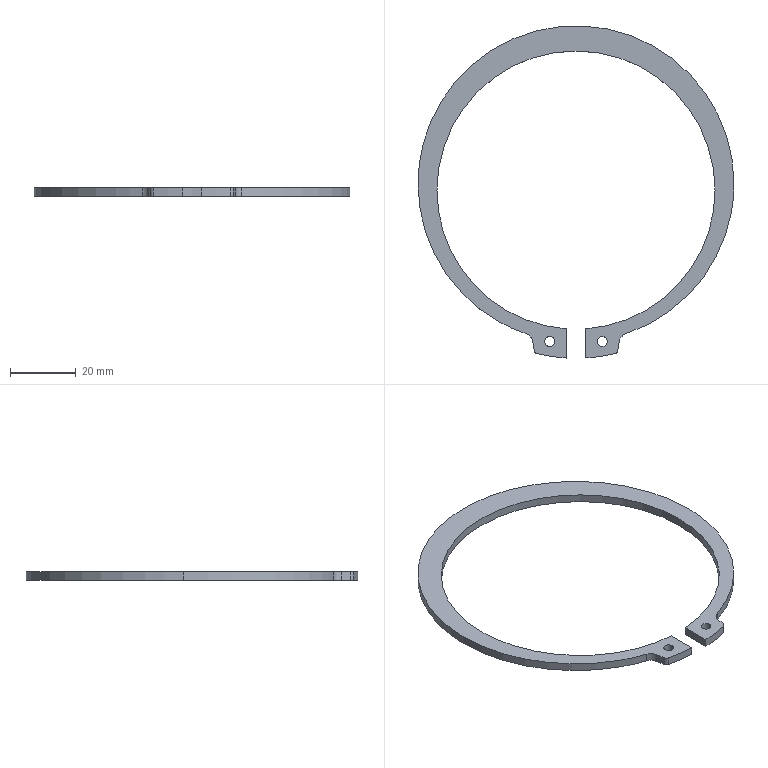Part | STEP file | PN_0045_Default<As Machined> | 1 solid | 22 faces | box 96 x 100.912 x 2.5 mm | volume 4237 mm3 | cylinder 16 | plane 6 | commonest cylinder face diameters 3 x4 84.5 x3 96 x3 2.4 x2 6 x2 102.2 x2
STEP:
#1=CARTESIAN_POINT('',(6.5,-47.91,-2.5));
#2=VERTEX_POINT('',#1);
#3=CARTESIAN_POINT('',(9.5,-47.91,-2.5));
#4=VERTEX_POINT('',#3);
#5=CARTESIAN_POINT('',(8.,-47.91,-2.5));
#6=DIRECTION('',(0.,0.,1.));
#7=AXIS2_PLACEMENT_3D('',#5,#6,$);
#8=CIRCLE('',#7,1.5);
#9=EDGE_CURVE('',#2,#4,#8,.T.);
#10=ORIENTED_EDGE('',*,*,#9,.F.);
#11=CARTESIAN_POINT('',(6.5,-47.91,0.));
#12=VERTEX_POINT('',#11);
#13=CARTESIAN_POINT('',(6.5,-47.91,-2.5));
#14=DIRECTION('',(0.,0.,1.));
#15=VECTOR('',#14,1.);
#16=LINE('',#13,#15);
#17=EDGE_CURVE('',#2,#12,#16,.T.);
#18=ORIENTED_EDGE('',*,*,#17,.T.);
#19=CARTESIAN_POINT('',(9.5,-47.91,0.));
#20=VERTEX_POINT('',#19);
#21=CARTESIAN_POINT('',(8.,-47.91,0.));
#22=DIRECTION('',(0.,0.,1.));
#23=AXIS2_PLACEMENT_3D('',#21,#22,$);
#24=CIRCLE('',#23,1.5);
#25=EDGE_CURVE('',#12,#20,#24,.T.);
#26=ORIENTED_EDGE('',*,*,#25,.T.);
#27=CARTESIAN_POINT('',(9.5,-47.91,-2.5));
#28=DIRECTION('',(0.,0.,1.));
#29=VECTOR('',#28,1.);
#30=LINE('',#27,#29);
#31=EDGE_CURVE('',#4,#20,#30,.T.);
#32=ORIENTED_EDGE('',*,*,#31,.F.);
#33=EDGE_LOOP('',(#10,#18,#26,#32));
#34=FACE_OUTER_BOUND('',#33,.T.);
#35=CARTESIAN_POINT('',(8.,-47.91,-2.5));
#36=DIRECTION('',(0.,0.,1.));
#37=DIRECTION('',(-1.,0.,0.));
#38=AXIS2_PLACEMENT_3D('',#35,#36,#37);
#39=CYLINDRICAL_SURFACE('',#38,1.5);
#40=ADVANCED_FACE('',(#34),#39,.F.);
#41=CARTESIAN_POINT('',(-11.757,-51.629,-2.5));
#42=VERTEX_POINT('',#41);
#43=CARTESIAN_POINT('',(-3.,-52.912,-2.5));
#44=VERTEX_POINT('',#43);
#45=CARTESIAN_POINT('',(-11.757,-51.629,-2.5));
#46=CARTESIAN_POINT('',(-10.032,-52.037,-2.5));
#47=CARTESIAN_POINT('',(-8.29,-52.37,-2.5));
#48=CARTESIAN_POINT('',(-6.534,-52.627,-2.5));
#49=CARTESIAN_POINT('',(-4.769,-52.808,-2.5));
#50=CARTESIAN_POINT('',(-3.,-52.912,-2.5));
#51=B_SPLINE_CURVE_WITH_KNOTS('',5,(#45,#46,#47,#48,#49,#50),.UNSPECIFIED.,.F.,.U.,(6,6),(0.,12.532),.UNSPECIFIED.);
#52=EDGE_CURVE('',#42,#44,#51,.T.);
#53=ORIENTED_EDGE('',*,*,#52,.F.);
#54=CARTESIAN_POINT('',(-12.662,-50.67,-2.5));
#55=VERTEX_POINT('',#54);
#56=CARTESIAN_POINT('',(-11.481,-50.461,-2.5));
#57=DIRECTION('',(0.,0.,-1.));
#58=AXIS2_PLACEMENT_3D('',#56,#57,$);
#59=CIRCLE('',#58,1.2);
#60=EDGE_CURVE('',#42,#55,#59,.T.);
#61=ORIENTED_EDGE('',*,*,#60,.T.);
#62=CARTESIAN_POINT('',(-13.157,-47.867,-2.5));
#63=VERTEX_POINT('',#62);
#64=CARTESIAN_POINT('',(-12.91,-49.269,-2.5));
#65=DIRECTION('',(0.1736,-0.9848,0.));
#66=VECTOR('',#65,1.);
#67=LINE('',#64,#66);
#68=EDGE_CURVE('',#63,#55,#67,.T.);
#69=ORIENTED_EDGE('',*,*,#68,.F.);
#70=CARTESIAN_POINT('',(-15.163,-45.542,-2.5));
#71=VERTEX_POINT('',#70);
#72=CARTESIAN_POINT('',(-13.157,-47.867,-2.5));
#73=CARTESIAN_POINT('',(-13.216,-47.533,-2.5));
#74=CARTESIAN_POINT('',(-13.322,-47.207,-2.5));
#75=CARTESIAN_POINT('',(-13.474,-46.899,-2.5));
#76=CARTESIAN_POINT('',(-13.841,-46.361,-2.5));
#77=CARTESIAN_POINT('',(-14.337,-45.94,-2.5));
#78=CARTESIAN_POINT('',(-14.596,-45.772,-2.5));
#79=CARTESIAN_POINT('',(-14.873,-45.639,-2.5));
#80=CARTESIAN_POINT('',(-15.163,-45.542,-2.5));
#81=B_SPLINE_CURVE_WITH_KNOTS('',5,(#72,#73,#74,#75,#76,#77,#78,#79,#80),.UNSPECIFIED.,.F.,.U.,(6,3,6),(0.,2.4,4.56),.UNSPECIFIED.);
#82=EDGE_CURVE('',#63,#71,#81,.T.);
#83=ORIENTED_EDGE('',*,*,#82,.T.);
#84=CARTESIAN_POINT('',(-48.,0.,-2.5));
#85=VERTEX_POINT('',#84);
#86=CARTESIAN_POINT('',(-48.,0.,-2.5));
#87=CARTESIAN_POINT('',(-48.,-4.412,-2.5));
#88=CARTESIAN_POINT('',(-47.493,-8.825,-2.5));
#89=CARTESIAN_POINT('',(-46.479,-13.159,-2.5));
#90=CARTESIAN_POINT('',(-43.473,-21.518,-2.5));
#91=CARTESIAN_POINT('',(-38.65,-28.977,-2.5));
#92=CARTESIAN_POINT('',(-35.818,-32.412,-2.5));
#93=CARTESIAN_POINT('',(-30.318,-37.703,-2.5));
#94=CARTESIAN_POINT('',(-23.91,-41.803,-2.5));
#95=CARTESIAN_POINT('',(-21.095,-43.291,-2.5));
#96=CARTESIAN_POINT('',(-18.17,-44.541,-2.5));
#97=CARTESIAN_POINT('',(-15.163,-45.542,-2.5));
#98=B_SPLINE_CURVE_WITH_KNOTS('',5,(#86,#87,#88,#89,#90,#91,#92,#93,#94,#95,#96,#97),.UNSPECIFIED.,.F.,.U.,(6,3,3,6),(0.,31.2,62.399,84.811),.UNSPECIFIED.);
#99=EDGE_CURVE('',#85,#71,#98,.T.);
#100=ORIENTED_EDGE('',*,*,#99,.F.);
#101=CARTESIAN_POINT('',(48.,0.,-2.5));
#102=VERTEX_POINT('',#101);
#103=CARTESIAN_POINT('',(48.,0.,-2.5));
#104=CARTESIAN_POINT('',(48.,4.412,-2.5));
#105=CARTESIAN_POINT('',(47.493,8.825,-2.5));
#106=CARTESIAN_POINT('',(46.479,13.159,-2.5));
#107=CARTESIAN_POINT('',(43.473,21.518,-2.5));
#108=CARTESIAN_POINT('',(38.65,28.977,-2.5));
#109=CARTESIAN_POINT('',(35.818,32.412,-2.5));
#110=CARTESIAN_POINT('',(29.416,38.57,-2.5));
#111=CARTESIAN_POINT('',(21.784,43.115,-2.5));
#112=CARTESIAN_POINT('',(17.722,44.937,-2.5));
#113=CARTESIAN_POINT('',(9.253,47.616,-2.5));
#114=CARTESIAN_POINT('',(0.3973,48.304,-2.5));
#115=CARTESIAN_POINT('',(-4.051,48.136,-2.5));
#116=CARTESIAN_POINT('',(-12.83,46.78,-2.5));
#117=CARTESIAN_POINT('',(-21.072,43.468,-2.5));
#118=CARTESIAN_POINT('',(-24.984,41.343,-2.5));
#119=CARTESIAN_POINT('',(-32.25,36.233,-2.5));
#120=CARTESIAN_POINT('',(-38.168,29.609,-2.5));
#121=CARTESIAN_POINT('',(-40.731,25.969,-2.5));
#122=CARTESIAN_POINT('',(-44.627,18.81,-2.5));
#123=CARTESIAN_POINT('',(-46.939,11.01,-2.5));
#124=CARTESIAN_POINT('',(-47.646,7.37,-2.5));
#125=CARTESIAN_POINT('',(-48.,3.685,-2.5));
#126=CARTESIAN_POINT('',(-48.,0.,-2.5));
#127=B_SPLINE_CURVE_WITH_KNOTS('',5,(#103,#104,#105,#106,#107,#108,#109,#110,#111,#112,#113,#114,#115,#116,#117,#118,#119,#120,#121,#122,#123,#124,#125,#126),.UNSPECIFIED.,.F.,.U.,(6,3,3,3,3,3,3,6),(0.,31.2,62.399,93.599,124.799,155.999,187.198,213.257),.UNSPECIFIED.);
#128=EDGE_CURVE('',#102,#85,#127,.T.);
#129=ORIENTED_EDGE('',*,*,#128,.F.);
#130=CARTESIAN_POINT('',(15.163,-45.542,-2.5));
#131=VERTEX_POINT('',#130);
#132=CARTESIAN_POINT('',(15.163,-45.542,-2.5));
#133=CARTESIAN_POINT('',(19.35,-44.148,-2.5));
#134=CARTESIAN_POINT('',(23.376,-42.273,-2.5));
#135=CARTESIAN_POINT('',(27.168,-39.942,-2.5));
#136=CARTESIAN_POINT('',(34.149,-34.449,-2.5));
#137=CARTESIAN_POINT('',(39.703,-27.516,-2.5));
#138=CARTESIAN_POINT('',(42.067,-23.745,-2.5));
#139=CARTESIAN_POINT('',(45.349,-16.855,-2.5));
#140=CARTESIAN_POINT('',(47.215,-9.48,-2.5));
#141=CARTESIAN_POINT('',(47.738,-6.339,-2.5));
#142=CARTESIAN_POINT('',(48.,-3.169,-2.5));
#143=CARTESIAN_POINT('',(48.,0.,-2.5));
#144=B_SPLINE_CURVE_WITH_KNOTS('',5,(#132,#133,#134,#135,#136,#137,#138,#139,#140,#141,#142,#143),.UNSPECIFIED.,.F.,.U.,(6,3,3,6),(0.,31.2,62.399,84.811),.UNSPECIFIED.);
#145=EDGE_CURVE('',#131,#102,#144,.T.);
#146=ORIENTED_EDGE('',*,*,#145,.F.);
#147=CARTESIAN_POINT('',(13.157,-47.867,-2.5));
#148=VERTEX_POINT('',#147);
#149=CARTESIAN_POINT('',(15.163,-45.542,-2.5));
#150=CARTESIAN_POINT('',(14.841,-45.649,-2.5));
#151=CARTESIAN_POINT('',(14.534,-45.802,-2.5));
#152=CARTESIAN_POINT('',(14.251,-45.997,-2.5));
#153=CARTESIAN_POINT('',(13.773,-46.44,-2.5));
#154=CARTESIAN_POINT('',(13.43,-46.992,-2.5));
#155=CARTESIAN_POINT('',(13.301,-47.272,-2.5));
#156=CARTESIAN_POINT('',(13.21,-47.567,-2.5));
#157=CARTESIAN_POINT('',(13.157,-47.867,-2.5));
#158=B_SPLINE_CURVE_WITH_KNOTS('',5,(#149,#150,#151,#152,#153,#154,#155,#156,#157),.UNSPECIFIED.,.F.,.U.,(6,3,6),(0.,2.4,4.56),.UNSPECIFIED.);
#159=EDGE_CURVE('',#131,#148,#158,.T.);
#160=ORIENTED_EDGE('',*,*,#159,.T.);
#161=CARTESIAN_POINT('',(12.662,-50.67,-2.5));
#162=VERTEX_POINT('',#161);
#163=CARTESIAN_POINT('',(12.91,-49.269,-2.5));
#164=DIRECTION('',(0.1736,0.9848,0.));
#165=VECTOR('',#164,1.);
#166=LINE('',#163,#165);
#167=EDGE_CURVE('',#162,#148,#166,.T.);
#168=ORIENTED_EDGE('',*,*,#167,.F.);
#169=CARTESIAN_POINT('',(11.757,-51.629,-2.5));
#170=VERTEX_POINT('',#169);
#171=CARTESIAN_POINT('',(11.481,-50.461,-2.5));
#172=DIRECTION('',(0.,0.,-1.));
#173=AXIS2_PLACEMENT_3D('',#171,#172,$);
#174=CIRCLE('',#173,1.2);
#175=EDGE_CURVE('',#162,#170,#174,.T.);
#176=ORIENTED_EDGE('',*,*,#175,.T.);
#177=CARTESIAN_POINT('',(3.,-52.912,-2.5));
#178=VERTEX_POINT('',#177);
#179=CARTESIAN_POINT('',(3.,-52.912,-2.5));
#180=CARTESIAN_POINT('',(4.769,-52.808,-2.5));
#181=CARTESIAN_POINT('',(6.534,-52.627,-2.5));
#182=CARTESIAN_POINT('',(8.29,-52.37,-2.5));
#183=CARTESIAN_POINT('',(10.032,-52.037,-2.5));
#184=CARTESIAN_POINT('',(11.757,-51.629,-2.5));
#185=B_SPLINE_CURVE_WITH_KNOTS('',5,(#179,#180,#181,#182,#183,#184),.UNSPECIFIED.,.F.,.U.,(6,6),(0.,12.532),.UNSPECIFIED.);
#186=EDGE_CURVE('',#178,#170,#185,.T.);
#187=ORIENTED_EDGE('',*,*,#186,.F.);
#188=CARTESIAN_POINT('',(3.,-44.043,-2.5));
#189=VERTEX_POINT('',#188);
#190=CARTESIAN_POINT('',(3.,-48.478,-2.5));
#191=DIRECTION('',(0.,-1.,0.));
#192=VECTOR('',#191,1.);
#193=LINE('',#190,#192);
#194=EDGE_CURVE('',#189,#178,#193,.T.);
#195=ORIENTED_EDGE('',*,*,#194,.F.);
#196=CARTESIAN_POINT('',(42.25,-1.9,-2.5));
#197=VERTEX_POINT('',#196);
#198=CARTESIAN_POINT('',(0.000000001,-1.9,-2.5));
#199=DIRECTION('',(0.,0.,-1.));
#200=AXIS2_PLACEMENT_3D('',#198,#199,$);
#201=CIRCLE('',#200,42.25);
#202=EDGE_CURVE('',#197,#189,#201,.T.);
#203=ORIENTED_EDGE('',*,*,#202,.F.);
#204=CARTESIAN_POINT('',(-42.25,-1.9,-2.5));
#205=VERTEX_POINT('',#204);
#206=CARTESIAN_POINT('',(0.,-1.9,-2.5));
#207=DIRECTION('',(0.,0.,-1.));
#208=AXIS2_PLACEMENT_3D('',#206,#207,$);
#209=CIRCLE('',#208,42.25);
#210=EDGE_CURVE('',#205,#197,#209,.T.);
#211=ORIENTED_EDGE('',*,*,#210,.F.);
#212=CARTESIAN_POINT('',(-3.,-44.043,-2.5));
#213=VERTEX_POINT('',#212);
#214=CARTESIAN_POINT('',(-0.000000001,-1.9,-2.5));
#215=DIRECTION('',(0.,0.,-1.));
#216=AXIS2_PLACEMENT_3D('',#214,#215,$);
#217=CIRCLE('',#216,42.25);
#218=EDGE_CURVE('',#213,#205,#217,.T.);
#219=ORIENTED_EDGE('',*,*,#218,.F.);
#220=CARTESIAN_POINT('',(-3.,-48.478,-2.5));
#221=DIRECTION('',(0.,1.,0.));
#222=VECTOR('',#221,1.);
#223=LINE('',#220,#222);
#224=EDGE_CURVE('',#44,#213,#223,.T.);
#225=ORIENTED_EDGE('',*,*,#224,.F.);
#226=EDGE_LOOP('',(#53,#61,#69,#83,#100,#129,#146,#160,#168,#176,#187,#195,#203,#211,#219,#225));
#227=FACE_OUTER_BOUND('',#226,.T.);
#228=CARTESIAN_POINT('',(9.5,-47.91,-2.5));
#229=CARTESIAN_POINT('',(9.5,-47.73,-2.5));
#230=CARTESIAN_POINT('',(9.473,-47.55,-2.5));
#231=CARTESIAN_POINT('',(9.419,-47.375,-2.5));
#232=CARTESIAN_POINT('',(9.26,-47.047,-2.5));
#233=CARTESIAN_POINT('',(9.012,-46.781,-2.5));
#234=CARTESIAN_POINT('',(8.869,-46.667,-2.5));
#235=CARTESIAN_POINT('',(8.553,-46.486,-2.5));
#236=CARTESIAN_POINT('',(8.198,-46.406,-2.5));
#237=CARTESIAN_POINT('',(8.016,-46.393,-2.5));
#238=CARTESIAN_POINT('',(7.653,-46.423,-2.5));
#239=CARTESIAN_POINT('',(7.315,-46.557,-2.5));
#240=CARTESIAN_POINT('',(7.157,-46.649,-2.5));
#241=CARTESIAN_POINT('',(6.874,-46.878,-2.5));
#242=CARTESIAN_POINT('',(6.671,-47.18,-2.5));
#243=CARTESIAN_POINT('',(6.593,-47.345,-2.5));
#244=CARTESIAN_POINT('',(6.528,-47.561,-2.5));
#245=CARTESIAN_POINT('',(6.505,-47.782,-2.5));
#246=CARTESIAN_POINT('',(6.502,-47.825,-2.5));
#247=CARTESIAN_POINT('',(6.5,-47.867,-2.5));
#248=CARTESIAN_POINT('',(6.5,-47.91,-2.5));
#249=B_SPLINE_CURVE_WITH_KNOTS('',5,(#228,#229,#230,#231,#232,#233,#234,#235,#236,#237,#238,#239,#240,#241,#242,#243,#244,#245,#246,#247,#248),.UNSPECIFIED.,.F.,.U.,(6,3,3,3,3,3,6),(0.,1.273,2.546,3.818,5.091,6.364,6.664),.UNSPECIFIED.);
#250=EDGE_CURVE('',#4,#2,#249,.T.);
#251=ORIENTED_EDGE('',*,*,#250,.T.);
#252=ORIENTED_EDGE('',*,*,#9,.T.);
#253=EDGE_LOOP('',(#251,#252));
#254=FACE_BOUND('',#253,.T.);
#255=CARTESIAN_POINT('',(-6.5,-47.91,-2.5));
#256=VERTEX_POINT('',#255);
#257=CARTESIAN_POINT('',(-9.5,-47.91,-2.5));
#258=VERTEX_POINT('',#257);
#259=CARTESIAN_POINT('',(-6.5,-47.91,-2.5));
#260=CARTESIAN_POINT('',(-6.5,-47.73,-2.5));
#261=CARTESIAN_POINT('',(-6.527,-47.55,-2.5));
#262=CARTESIAN_POINT('',(-6.581,-47.375,-2.5));
#263=CARTESIAN_POINT('',(-6.74,-47.047,-2.5));
#264=CARTESIAN_POINT('',(-6.988,-46.781,-2.5));
#265=CARTESIAN_POINT('',(-7.131,-46.667,-2.5));
#266=CARTESIAN_POINT('',(-7.447,-46.486,-2.5));
#267=CARTESIAN_POINT('',(-7.802,-46.406,-2.5));
#268=CARTESIAN_POINT('',(-7.984,-46.393,-2.5));
#269=CARTESIAN_POINT('',(-8.347,-46.423,-2.5));
#270=CARTESIAN_POINT('',(-8.685,-46.557,-2.5));
#271=CARTESIAN_POINT('',(-8.843,-46.649,-2.5));
#272=CARTESIAN_POINT('',(-9.126,-46.878,-2.5));
#273=CARTESIAN_POINT('',(-9.329,-47.18,-2.5));
#274=CARTESIAN_POINT('',(-9.407,-47.345,-2.5));
#275=CARTESIAN_POINT('',(-9.472,-47.561,-2.5));
#276=CARTESIAN_POINT('',(-9.495,-47.782,-2.5));
#277=CARTESIAN_POINT('',(-9.498,-47.825,-2.5));
#278=CARTESIAN_POINT('',(-9.5,-47.867,-2.5));
#279=CARTESIAN_POINT('',(-9.5,-47.91,-2.5));
#280=B_SPLINE_CURVE_WITH_KNOTS('',5,(#259,#260,#261,#262,#263,#264,#265,#266,#267,#268,#269,#270,#271,#272,#273,#274,#275,#276,#277,#278,#279),.UNSPECIFIED.,.F.,.U.,(6,3,3,3,3,3,6),(0.,1.273,2.546,3.818,5.091,6.364,6.664),.UNSPECIFIED.);
#281=EDGE_CURVE('',#256,#258,#280,.T.);
#282=ORIENTED_EDGE('',*,*,#281,.T.);
#283=CARTESIAN_POINT('',(-9.5,-47.91,-2.5));
#284=CARTESIAN_POINT('',(-9.5,-48.09,-2.5));
#285=CARTESIAN_POINT('',(-9.473,-48.27,-2.5));
#286=CARTESIAN_POINT('',(-9.419,-48.444,-2.5));
#287=CARTESIAN_POINT('',(-9.26,-48.772,-2.5));
#288=CARTESIAN_POINT('',(-9.012,-49.039,-2.5));
#289=CARTESIAN_POINT('',(-8.869,-49.152,-2.5));
#290=CARTESIAN_POINT('',(-8.553,-49.333,-2.5));
#291=CARTESIAN_POINT('',(-8.198,-49.413,-2.5));
#292=CARTESIAN_POINT('',(-8.016,-49.426,-2.5));
#293=CARTESIAN_POINT('',(-7.653,-49.397,-2.5));
#294=CARTESIAN_POINT('',(-7.315,-49.262,-2.5));
#295=CARTESIAN_POINT('',(-7.157,-49.17,-2.5));
#296=CARTESIAN_POINT('',(-6.874,-48.941,-2.5));
#297=CARTESIAN_POINT('',(-6.671,-48.639,-2.5));
#298=CARTESIAN_POINT('',(-6.593,-48.474,-2.5));
#299=CARTESIAN_POINT('',(-6.528,-48.258,-2.5));
#300=CARTESIAN_POINT('',(-6.505,-48.037,-2.5));
#301=CARTESIAN_POINT('',(-6.502,-47.995,-2.5));
#302=CARTESIAN_POINT('',(-6.5,-47.952,-2.5));
#303=CARTESIAN_POINT('',(-6.5,-47.91,-2.5));
#304=B_SPLINE_CURVE_WITH_KNOTS('',5,(#283,#284,#285,#286,#287,#288,#289,#290,#291,#292,#293,#294,#295,#296,#297,#298,#299,#300,#301,#302,#303),.UNSPECIFIED.,.F.,.U.,(6,3,3,3,3,3,6),(0.,1.273,2.546,3.818,5.091,6.364,6.664),.UNSPECIFIED.);
#305=EDGE_CURVE('',#258,#256,#304,.T.);
#306=ORIENTED_EDGE('',*,*,#305,.T.);
#307=EDGE_LOOP('',(#282,#306));
#308=FACE_BOUND('',#307,.T.);
#309=CARTESIAN_POINT('',(0.,-1.9,-2.5));
#310=DIRECTION('',(0.,0.,-1.));
#311=DIRECTION('',(-1.,0.,0.));
#312=AXIS2_PLACEMENT_3D('',#309,#310,#311);
#313=PLANE('',#312);
#314=ADVANCED_FACE('',(#227,#254,#308),#313,.T.);
#315=ORIENTED_EDGE('',*,*,#17,.F.);
#316=ORIENTED_EDGE('',*,*,#250,.F.);
#317=ORIENTED_EDGE('',*,*,#31,.T.);
#318=CARTESIAN_POINT('',(8.,-47.91,0.));
#319=DIRECTION('',(0.,0.,1.));
#320=AXIS2_PLACEMENT_3D('',#318,#319,$);
#321=CIRCLE('',#320,1.5);
#322=EDGE_CURVE('',#20,#12,#321,.T.);
#323=ORIENTED_EDGE('',*,*,#322,.T.);
#324=EDGE_LOOP('',(#315,#316,#317,#323));
#325=FACE_OUTER_BOUND('',#324,.T.);
#326=CARTESIAN_POINT('',(8.,-47.91,-2.5));
#327=DIRECTION('',(0.,0.,1.));
#328=DIRECTION('',(1.,0.,0.));
#329=AXIS2_PLACEMENT_3D('',#326,#327,#328);
#330=CYLINDRICAL_SURFACE('',#329,1.5);
#331=ADVANCED_FACE('',(#325),#330,.F.);
#332=CARTESIAN_POINT('',(15.163,-45.542,0.));
#333=VERTEX_POINT('',#332);
#334=CARTESIAN_POINT('',(48.,0.,0.));
#335=VERTEX_POINT('',#334);
#336=CARTESIAN_POINT('',(15.163,-45.542,0.));
#337=CARTESIAN_POINT('',(19.35,-44.148,0.));
#338=CARTESIAN_POINT('',(23.376,-42.273,0.));
#339=CARTESIAN_POINT('',(27.168,-39.942,0.));
#340=CARTESIAN_POINT('',(34.149,-34.449,0.));
#341=CARTESIAN_POINT('',(39.703,-27.516,0.));
#342=CARTESIAN_POINT('',(42.067,-23.745,0.));
#343=CARTESIAN_POINT('',(45.349,-16.855,0.));
#344=CARTESIAN_POINT('',(47.215,-9.48,0.));
#345=CARTESIAN_POINT('',(47.738,-6.339,0.));
#346=CARTESIAN_POINT('',(48.,-3.169,0.));
#347=CARTESIAN_POINT('',(48.,0.,0.));
#348=B_SPLINE_CURVE_WITH_KNOTS('',5,(#336,#337,#338,#339,#340,#341,#342,#343,#344,#345,#346,#347),.UNSPECIFIED.,.F.,.U.,(6,3,3,6),(0.,31.2,62.399,84.811),.UNSPECIFIED.);
#349=EDGE_CURVE('',#333,#335,#348,.T.);
#350=ORIENTED_EDGE('',*,*,#349,.T.);
#351=CARTESIAN_POINT('',(-48.,0.,0.));
#352=VERTEX_POINT('',#351);
#353=CARTESIAN_POINT('',(48.,0.,0.));
#354=CARTESIAN_POINT('',(48.,4.412,0.));
#355=CARTESIAN_POINT('',(47.493,8.825,0.));
#356=CARTESIAN_POINT('',(46.479,13.159,0.));
#357=CARTESIAN_POINT('',(43.473,21.518,0.));
#358=CARTESIAN_POINT('',(38.65,28.977,0.));
#359=CARTESIAN_POINT('',(35.818,32.412,0.));
#360=CARTESIAN_POINT('',(29.416,38.57,0.));
#361=CARTESIAN_POINT('',(21.784,43.115,0.));
#362=CARTESIAN_POINT('',(17.722,44.937,0.));
#363=CARTESIAN_POINT('',(9.253,47.616,0.));
#364=CARTESIAN_POINT('',(0.3973,48.304,0.));
#365=CARTESIAN_POINT('',(-4.051,48.136,0.));
#366=CARTESIAN_POINT('',(-12.83,46.78,0.));
#367=CARTESIAN_POINT('',(-21.072,43.468,0.));
#368=CARTESIAN_POINT('',(-24.984,41.343,0.));
#369=CARTESIAN_POINT('',(-32.25,36.233,0.));
#370=CARTESIAN_POINT('',(-38.168,29.609,0.));
#371=CARTESIAN_POINT('',(-40.731,25.969,0.));
#372=CARTESIAN_POINT('',(-44.627,18.81,0.));
#373=CARTESIAN_POINT('',(-46.939,11.01,0.));
#374=CARTESIAN_POINT('',(-47.646,7.37,0.));
#375=CARTESIAN_POINT('',(-48.,3.685,0.));
#376=CARTESIAN_POINT('',(-48.,0.,0.));
#377=B_SPLINE_CURVE_WITH_KNOTS('',5,(#353,#354,#355,#356,#357,#358,#359,#360,#361,#362,#363,#364,#365,#366,#367,#368,#369,#370,#371,#372,#373,#374,#375,#376),.UNSPECIFIED.,.F.,.U.,(6,3,3,3,3,3,3,6),(0.,31.2,62.399,93.599,124.799,155.999,187.198,213.257),.UNSPECIFIED.);
#378=EDGE_CURVE('',#335,#352,#377,.T.);
#379=ORIENTED_EDGE('',*,*,#378,.T.);
#380=CARTESIAN_POINT('',(-15.163,-45.542,0.));
#381=VERTEX_POINT('',#380);
#382=CARTESIAN_POINT('',(-48.,0.,0.));
#383=CARTESIAN_POINT('',(-48.,-4.412,0.));
#384=CARTESIAN_POINT('',(-47.493,-8.825,0.));
#385=CARTESIAN_POINT('',(-46.479,-13.159,0.));
#386=CARTESIAN_POINT('',(-43.473,-21.518,0.));
#387=CARTESIAN_POINT('',(-38.65,-28.977,0.));
#388=CARTESIAN_POINT('',(-35.818,-32.412,0.));
#389=CARTESIAN_POINT('',(-30.318,-37.703,0.));
#390=CARTESIAN_POINT('',(-23.91,-41.803,0.));
#391=CARTESIAN_POINT('',(-21.095,-43.291,0.));
#392=CARTESIAN_POINT('',(-18.17,-44.541,0.));
#393=CARTESIAN_POINT('',(-15.163,-45.542,0.));
#394=B_SPLINE_CURVE_WITH_KNOTS('',5,(#382,#383,#384,#385,#386,#387,#388,#389,#390,#391,#392,#393),.UNSPECIFIED.,.F.,.U.,(6,3,3,6),(0.,31.2,62.399,84.811),.UNSPECIFIED.);
#395=EDGE_CURVE('',#352,#381,#394,.T.);
#396=ORIENTED_EDGE('',*,*,#395,.T.);
#397=CARTESIAN_POINT('',(-13.157,-47.867,0.));
#398=VERTEX_POINT('',#397);
#399=CARTESIAN_POINT('',(-16.111,-48.388,0.));
#400=DIRECTION('',(0.,0.,-1.));
#401=AXIS2_PLACEMENT_3D('',#399,#400,$);
#402=CIRCLE('',#401,3.);
#403=EDGE_CURVE('',#381,#398,#402,.T.);
#404=ORIENTED_EDGE('',*,*,#403,.T.);
#405=CARTESIAN_POINT('',(-12.662,-50.67,0.));
#406=VERTEX_POINT('',#405);
#407=CARTESIAN_POINT('',(-12.91,-49.269,0.));
#408=DIRECTION('',(0.1736,-0.9848,0.));
#409=VECTOR('',#408,1.);
#410=LINE('',#407,#409);
#411=EDGE_CURVE('',#398,#406,#410,.T.);
#412=ORIENTED_EDGE('',*,*,#411,.T.);
#413=CARTESIAN_POINT('',(-11.757,-51.629,0.));
#414=VERTEX_POINT('',#413);
#415=CARTESIAN_POINT('',(-12.662,-50.67,0.));
#416=CARTESIAN_POINT('',(-12.635,-50.828,0.));
#417=CARTESIAN_POINT('',(-12.58,-50.982,0.));
#418=CARTESIAN_POINT('',(-12.5,-51.125,0.));
#419=CARTESIAN_POINT('',(-12.322,-51.346,0.));
#420=CARTESIAN_POINT('',(-12.09,-51.505,0.));
#421=CARTESIAN_POINT('',(-11.984,-51.56,0.));
#422=CARTESIAN_POINT('',(-11.872,-51.602,0.));
#423=CARTESIAN_POINT('',(-11.757,-51.629,0.));
#424=B_SPLINE_CURVE_WITH_KNOTS('',5,(#415,#416,#417,#418,#419,#420,#421,#422,#423),.UNSPECIFIED.,.F.,.U.,(6,3,6),(0.,1.138,1.976),.UNSPECIFIED.);
#425=EDGE_CURVE('',#406,#414,#424,.T.);
#426=ORIENTED_EDGE('',*,*,#425,.T.);
#427=CARTESIAN_POINT('',(-3.,-52.912,0.));
#428=VERTEX_POINT('',#427);
#429=CARTESIAN_POINT('',(-11.757,-51.629,0.));
#430=CARTESIAN_POINT('',(-10.032,-52.037,0.));
#431=CARTESIAN_POINT('',(-8.29,-52.37,0.));
#432=CARTESIAN_POINT('',(-6.534,-52.627,0.));
#433=CARTESIAN_POINT('',(-4.769,-52.808,0.));
#434=CARTESIAN_POINT('',(-3.,-52.912,0.));
#435=B_SPLINE_CURVE_WITH_KNOTS('',5,(#429,#430,#431,#432,#433,#434),.UNSPECIFIED.,.F.,.U.,(6,6),(0.,12.532),.UNSPECIFIED.);
#436=EDGE_CURVE('',#414,#428,#435,.T.);
#437=ORIENTED_EDGE('',*,*,#436,.T.);
#438=CARTESIAN_POINT('',(-3.,-44.043,0.));
#439=VERTEX_POINT('',#438);
#440=CARTESIAN_POINT('',(-3.,-48.478,0.));
#441=DIRECTION('',(0.,1.,0.));
#442=VECTOR('',#441,1.);
#443=LINE('',#440,#442);
#444=EDGE_CURVE('',#428,#439,#443,.T.);
#445=ORIENTED_EDGE('',*,*,#444,.T.);
#446=CARTESIAN_POINT('',(-42.25,-1.9,0.));
#447=VERTEX_POINT('',#446);
#448=CARTESIAN_POINT('',(-0.000000001,-1.9,0.));
#449=DIRECTION('',(0.,0.,-1.));
#450=AXIS2_PLACEMENT_3D('',#448,#449,$);
#451=CIRCLE('',#450,42.25);
#452=EDGE_CURVE('',#439,#447,#451,.T.);
#453=ORIENTED_EDGE('',*,*,#452,.T.);
#454=CARTESIAN_POINT('',(42.25,-1.9,0.));
#455=VERTEX_POINT('',#454);
#456=CARTESIAN_POINT('',(0.,-1.9,0.));
#457=DIRECTION('',(0.,0.,-1.));
#458=AXIS2_PLACEMENT_3D('',#456,#457,$);
#459=CIRCLE('',#458,42.25);
#460=EDGE_CURVE('',#447,#455,#459,.T.);
#461=ORIENTED_EDGE('',*,*,#460,.T.);
#462=CARTESIAN_POINT('',(3.,-44.043,0.));
#463=VERTEX_POINT('',#462);
#464=CARTESIAN_POINT('',(0.000000001,-1.9,0.));
#465=DIRECTION('',(0.,0.,-1.));
#466=AXIS2_PLACEMENT_3D('',#464,#465,$);
#467=CIRCLE('',#466,42.25);
#468=EDGE_CURVE('',#455,#463,#467,.T.);
#469=ORIENTED_EDGE('',*,*,#468,.T.);
#470=CARTESIAN_POINT('',(3.,-52.912,0.));
#471=VERTEX_POINT('',#470);
#472=CARTESIAN_POINT('',(3.,-48.478,0.));
#473=DIRECTION('',(0.,-1.,0.));
#474=VECTOR('',#473,1.);
#475=LINE('',#472,#474);
#476=EDGE_CURVE('',#463,#471,#475,.T.);
#477=ORIENTED_EDGE('',*,*,#476,.T.);
#478=CARTESIAN_POINT('',(11.757,-51.629,0.));
#479=VERTEX_POINT('',#478);
#480=CARTESIAN_POINT('',(3.,-52.912,0.));
#481=CARTESIAN_POINT('',(4.769,-52.808,0.));
#482=CARTESIAN_POINT('',(6.534,-52.627,0.));
#483=CARTESIAN_POINT('',(8.29,-52.37,0.));
#484=CARTESIAN_POINT('',(10.032,-52.037,0.));
#485=CARTESIAN_POINT('',(11.757,-51.629,0.));
#486=B_SPLINE_CURVE_WITH_KNOTS('',5,(#480,#481,#482,#483,#484,#485),.UNSPECIFIED.,.F.,.U.,(6,6),(0.,12.532),.UNSPECIFIED.);
#487=EDGE_CURVE('',#471,#479,#486,.T.);
#488=ORIENTED_EDGE('',*,*,#487,.T.);
#489=CARTESIAN_POINT('',(12.662,-50.67,0.));
#490=VERTEX_POINT('',#489);
#491=CARTESIAN_POINT('',(11.757,-51.629,0.));
#492=CARTESIAN_POINT('',(11.913,-51.592,0.));
#493=CARTESIAN_POINT('',(12.064,-51.529,0.));
#494=CARTESIAN_POINT('',(12.202,-51.441,0.));
#495=CARTESIAN_POINT('',(12.412,-51.25,0.));
#496=CARTESIAN_POINT('',(12.558,-51.01,0.));
#497=CARTESIAN_POINT('',(12.607,-50.9,0.));
#498=CARTESIAN_POINT('',(12.642,-50.786,0.));
#499=CARTESIAN_POINT('',(12.662,-50.67,0.));
#500=B_SPLINE_CURVE_WITH_KNOTS('',5,(#491,#492,#493,#494,#495,#496,#497,#498,#499),.UNSPECIFIED.,.F.,.U.,(6,3,6),(0.,1.138,1.976),.UNSPECIFIED.);
#501=EDGE_CURVE('',#479,#490,#500,.T.);
#502=ORIENTED_EDGE('',*,*,#501,.T.);
#503=CARTESIAN_POINT('',(13.157,-47.867,0.));
#504=VERTEX_POINT('',#503);
#505=CARTESIAN_POINT('',(12.91,-49.269,0.));
#506=DIRECTION('',(0.1736,0.9848,0.));
#507=VECTOR('',#506,1.);
#508=LINE('',#505,#507);
#509=EDGE_CURVE('',#490,#504,#508,.T.);
#510=ORIENTED_EDGE('',*,*,#509,.T.);
#511=CARTESIAN_POINT('',(16.111,-48.388,0.));
#512=DIRECTION('',(0.,0.,-1.));
#513=AXIS2_PLACEMENT_3D('',#511,#512,$);
#514=CIRCLE('',#513,3.);
#515=EDGE_CURVE('',#504,#333,#514,.T.);
#516=ORIENTED_EDGE('',*,*,#515,.T.);
#517=EDGE_LOOP('',(#350,#379,#396,#404,#412,#426,#437,#445,#453,#461,#469,#477,#488,#502,#510,#516));
#518=FACE_OUTER_BOUND('',#517,.T.);
#519=ORIENTED_EDGE('',*,*,#322,.F.);
#520=ORIENTED_EDGE('',*,*,#25,.F.);
#521=EDGE_LOOP('',(#519,#520));
#522=FACE_BOUND('',#521,.T.);
#523=CARTESIAN_POINT('',(-6.5,-47.91,0.));
#524=VERTEX_POINT('',#523);
#525=CARTESIAN_POINT('',(-9.5,-47.91,0.));
#526=VERTEX_POINT('',#525);
#527=CARTESIAN_POINT('',(-6.5,-47.91,0.));
#528=CARTESIAN_POINT('',(-6.5,-47.73,0.));
#529=CARTESIAN_POINT('',(-6.527,-47.55,0.));
#530=CARTESIAN_POINT('',(-6.581,-47.375,0.));
#531=CARTESIAN_POINT('',(-6.74,-47.047,0.));
#532=CARTESIAN_POINT('',(-6.988,-46.781,0.));
#533=CARTESIAN_POINT('',(-7.131,-46.667,0.));
#534=CARTESIAN_POINT('',(-7.447,-46.486,0.));
#535=CARTESIAN_POINT('',(-7.802,-46.406,0.));
#536=CARTESIAN_POINT('',(-7.984,-46.393,0.));
#537=CARTESIAN_POINT('',(-8.347,-46.423,0.));
#538=CARTESIAN_POINT('',(-8.685,-46.557,0.));
#539=CARTESIAN_POINT('',(-8.843,-46.649,0.));
#540=CARTESIAN_POINT('',(-9.126,-46.878,0.));
#541=CARTESIAN_POINT('',(-9.329,-47.18,0.));
#542=CARTESIAN_POINT('',(-9.407,-47.345,0.));
#543=CARTESIAN_POINT('',(-9.472,-47.561,0.));
#544=CARTESIAN_POINT('',(-9.495,-47.782,0.));
#545=CARTESIAN_POINT('',(-9.498,-47.825,0.));
#546=CARTESIAN_POINT('',(-9.5,-47.867,0.));
#547=CARTESIAN_POINT('',(-9.5,-47.91,0.));
#548=B_SPLINE_CURVE_WITH_KNOTS('',5,(#527,#528,#529,#530,#531,#532,#533,#534,#535,#536,#537,#538,#539,#540,#541,#542,#543,#544,#545,#546,#547),.UNSPECIFIED.,.F.,.U.,(6,3,3,3,3,3,6),(0.,1.273,2.546,3.818,5.091,6.364,6.664),.UNSPECIFIED.);
#549=EDGE_CURVE('',#524,#526,#548,.T.);
#550=ORIENTED_EDGE('',*,*,#549,.F.);
#551=CARTESIAN_POINT('',(-9.5,-47.91,0.));
#552=CARTESIAN_POINT('',(-9.5,-48.09,0.));
#553=CARTESIAN_POINT('',(-9.473,-48.27,0.));
#554=CARTESIAN_POINT('',(-9.419,-48.444,0.));
#555=CARTESIAN_POINT('',(-9.26,-48.772,0.));
#556=CARTESIAN_POINT('',(-9.012,-49.039,0.));
#557=CARTESIAN_POINT('',(-8.869,-49.152,0.));
#558=CARTESIAN_POINT('',(-8.553,-49.333,0.));
#559=CARTESIAN_POINT('',(-8.198,-49.413,0.));
#560=CARTESIAN_POINT('',(-8.016,-49.426,0.));
#561=CARTESIAN_POINT('',(-7.653,-49.397,0.));
#562=CARTESIAN_POINT('',(-7.315,-49.262,0.));
#563=CARTESIAN_POINT('',(-7.157,-49.17,0.));
#564=CARTESIAN_POINT('',(-6.874,-48.941,0.));
#565=CARTESIAN_POINT('',(-6.671,-48.639,0.));
#566=CARTESIAN_POINT('',(-6.593,-48.474,0.));
#567=CARTESIAN_POINT('',(-6.528,-48.258,0.));
#568=CARTESIAN_POINT('',(-6.505,-48.037,0.));
#569=CARTESIAN_POINT('',(-6.502,-47.995,0.));
#570=CARTESIAN_POINT('',(-6.5,-47.952,0.));
#571=CARTESIAN_POINT('',(-6.5,-47.91,0.));
#572=B_SPLINE_CURVE_WITH_KNOTS('',5,(#551,#552,#553,#554,#555,#556,#557,#558,#559,#560,#561,#562,#563,#564,#565,#566,#567,#568,#569,#570,#571),.UNSPECIFIED.,.F.,.U.,(6,3,3,3,3,3,6),(0.,1.273,2.546,3.818,5.091,6.364,6.664),.UNSPECIFIED.);
#573=EDGE_CURVE('',#526,#524,#572,.T.);
#574=ORIENTED_EDGE('',*,*,#573,.F.);
#575=EDGE_LOOP('',(#550,#574));
#576=FACE_BOUND('',#575,.T.);
#577=CARTESIAN_POINT('',(0.,-1.9,0.));
#578=DIRECTION('',(0.,0.,-1.));
#579=DIRECTION('',(-1.,0.,0.));
#580=AXIS2_PLACEMENT_3D('',#577,#578,#579);
#581=PLANE('',#580);
#582=ADVANCED_FACE('',(#518,#522,#576),#581,.F.);
#583=ORIENTED_EDGE('',*,*,#436,.F.);
#584=CARTESIAN_POINT('',(-11.757,-51.629,-2.5));
#585=DIRECTION('',(0.,0.,1.));
#586=VECTOR('',#585,1.);
#587=LINE('',#584,#586);
#588=EDGE_CURVE('',#414,#42,#587,.F.);
#589=ORIENTED_EDGE('',*,*,#588,.T.);
#590=ORIENTED_EDGE('',*,*,#52,.T.);
#591=CARTESIAN_POINT('',(-3.,-52.912,-2.5));
#592=DIRECTION('',(0.,0.,1.));
#593=VECTOR('',#592,1.);
#594=LINE('',#591,#593);
#595=EDGE_CURVE('',#44,#428,#594,.T.);
#596=ORIENTED_EDGE('',*,*,#595,.T.);
#597=EDGE_LOOP('',(#583,#589,#590,#596));
#598=FACE_OUTER_BOUND('',#597,.T.);
#599=CARTESIAN_POINT('',(0.,-1.9,-2.5));
#600=DIRECTION('',(0.,0.,1.));
#601=DIRECTION('',(-1.,0.,0.));
#602=AXIS2_PLACEMENT_3D('',#599,#600,#601);
#603=CYLINDRICAL_SURFACE('',#602,51.1);
#604=ADVANCED_FACE('',(#598),#603,.T.);
#605=ORIENTED_EDGE('',*,*,#60,.F.);
#606=ORIENTED_EDGE('',*,*,#588,.F.);
#607=ORIENTED_EDGE('',*,*,#425,.F.);
#608=CARTESIAN_POINT('',(-12.662,-50.67,-2.5));
#609=DIRECTION('',(0.,0.,1.));
#610=VECTOR('',#609,1.);
#611=LINE('',#608,#610);
#612=EDGE_CURVE('',#55,#406,#611,.T.);
#613=ORIENTED_EDGE('',*,*,#612,.F.);
#614=EDGE_LOOP('',(#605,#606,#607,#613));
#615=FACE_OUTER_BOUND('',#614,.T.);
#616=CARTESIAN_POINT('',(-11.481,-50.461,-2.5));
#617=DIRECTION('',(0.,0.,1.));
#618=DIRECTION('',(-1.,0.,0.));
#619=AXIS2_PLACEMENT_3D('',#616,#617,#618);
#620=CYLINDRICAL_SURFACE('',#619,1.2);
#621=ADVANCED_FACE('',(#615),#620,.T.);
#622=ORIENTED_EDGE('',*,*,#411,.F.);
#623=CARTESIAN_POINT('',(-13.157,-47.867,-1.25));
#624=DIRECTION('',(0.,0.,-1.));
#625=VECTOR('',#624,1.);
#626=LINE('',#623,#625);
#627=EDGE_CURVE('',#398,#63,#626,.T.);
#628=ORIENTED_EDGE('',*,*,#627,.T.);
#629=ORIENTED_EDGE('',*,*,#68,.T.);
#630=ORIENTED_EDGE('',*,*,#612,.T.);
#631=EDGE_LOOP('',(#622,#628,#629,#630));
#632=FACE_OUTER_BOUND('',#631,.T.);
#633=CARTESIAN_POINT('',(-13.473,-46.07,-2.5));
#634=DIRECTION('',(-0.9848,-0.1736,0.));
#635=DIRECTION('',(0.1736,-0.9848,0.));
#636=AXIS2_PLACEMENT_3D('',#633,#634,#635);
#637=PLANE('',#636);
#638=ADVANCED_FACE('',(#632),#637,.T.);
#639=ORIENTED_EDGE('',*,*,#82,.F.);
#640=ORIENTED_EDGE('',*,*,#627,.F.);
#641=ORIENTED_EDGE('',*,*,#403,.F.);
#642=CARTESIAN_POINT('',(-15.163,-45.542,-2.5));
#643=DIRECTION('',(0.,0.,1.));
#644=VECTOR('',#643,1.);
#645=LINE('',#642,#644);
#646=EDGE_CURVE('',#71,#381,#645,.T.);
#647=ORIENTED_EDGE('',*,*,#646,.F.);
#648=EDGE_LOOP('',(#639,#640,#641,#647));
#649=FACE_OUTER_BOUND('',#648,.T.);
#650=CARTESIAN_POINT('',(-16.111,-48.388,-2.5));
#651=DIRECTION('',(0.,0.,1.));
#652=DIRECTION('',(1.,0.,0.));
#653=AXIS2_PLACEMENT_3D('',#650,#651,#652);
#654=CYLINDRICAL_SURFACE('',#653,3.);
#655=ADVANCED_FACE('',(#649),#654,.F.);
#656=CARTESIAN_POINT('',(-48.,0.,-2.5));
#657=DIRECTION('',(0.,0.,1.));
#658=VECTOR('',#657,1.);
#659=LINE('',#656,#658);
#660=EDGE_CURVE('',#85,#352,#659,.T.);
#661=ORIENTED_EDGE('',*,*,#660,.F.);
#662=ORIENTED_EDGE('',*,*,#99,.T.);
#663=ORIENTED_EDGE('',*,*,#646,.T.);
#664=ORIENTED_EDGE('',*,*,#395,.F.);
#665=EDGE_LOOP('',(#661,#662,#663,#664));
#666=FACE_OUTER_BOUND('',#665,.T.);
#667=CARTESIAN_POINT('',(0.,0.,-2.5));
#668=DIRECTION('',(0.,0.,1.));
#669=DIRECTION('',(-1.,0.,0.));
#670=AXIS2_PLACEMENT_3D('',#667,#668,#669);
#671=CYLINDRICAL_SURFACE('',#670,48.);
#672=ADVANCED_FACE('',(#666),#671,.T.);
#673=ORIENTED_EDGE('',*,*,#128,.T.);
#674=ORIENTED_EDGE('',*,*,#660,.T.);
#675=ORIENTED_EDGE('',*,*,#378,.F.);
#676=CARTESIAN_POINT('',(48.,0.,-2.5));
#677=DIRECTION('',(0.,0.,1.));
#678=VECTOR('',#677,1.);
#679=LINE('',#676,#678);
#680=EDGE_CURVE('',#102,#335,#679,.T.);
#681=ORIENTED_EDGE('',*,*,#680,.F.);
#682=EDGE_LOOP('',(#673,#674,#675,#681));
#683=FACE_OUTER_BOUND('',#682,.T.);
#684=CARTESIAN_POINT('',(0.,0.,-2.5));
#685=DIRECTION('',(0.,0.,1.));
#686=DIRECTION('',(1.,0.,0.));
#687=AXIS2_PLACEMENT_3D('',#684,#685,#686);
#688=CYLINDRICAL_SURFACE('',#687,48.);
#689=ADVANCED_FACE('',(#683),#688,.T.);
#690=ORIENTED_EDGE('',*,*,#145,.T.);
#691=ORIENTED_EDGE('',*,*,#680,.T.);
#692=ORIENTED_EDGE('',*,*,#349,.F.);
#693=CARTESIAN_POINT('',(15.163,-45.542,-2.5));
#694=DIRECTION('',(0.,0.,1.));
#695=VECTOR('',#694,1.);
#696=LINE('',#693,#695);
#697=EDGE_CURVE('',#333,#131,#696,.F.);
#698=ORIENTED_EDGE('',*,*,#697,.T.);
#699=EDGE_LOOP('',(#690,#691,#692,#698));
#700=FACE_OUTER_BOUND('',#699,.T.);
#701=CARTESIAN_POINT('',(0.,0.,-2.5));
#702=DIRECTION('',(0.,0.,1.));
#703=DIRECTION('',(-1.,0.,0.));
#704=AXIS2_PLACEMENT_3D('',#701,#702,#703);
#705=CYLINDRICAL_SURFACE('',#704,48.);
#706=ADVANCED_FACE('',(#700),#705,.T.);
#707=ORIENTED_EDGE('',*,*,#159,.F.);
#708=ORIENTED_EDGE('',*,*,#697,.F.);
#709=ORIENTED_EDGE('',*,*,#515,.F.);
#710=CARTESIAN_POINT('',(13.157,-47.867,-2.5));
#711=DIRECTION('',(0.,0.,1.));
#712=VECTOR('',#711,1.);
#713=LINE('',#710,#712);
#714=EDGE_CURVE('',#148,#504,#713,.T.);
#715=ORIENTED_EDGE('',*,*,#714,.F.);
#716=EDGE_LOOP('',(#707,#708,#709,#715));
#717=FACE_OUTER_BOUND('',#716,.T.);
#718=CARTESIAN_POINT('',(16.111,-48.388,-2.5));
#719=DIRECTION('',(0.,0.,1.));
#720=DIRECTION('',(1.,0.,0.));
#721=AXIS2_PLACEMENT_3D('',#718,#719,#720);
#722=CYLINDRICAL_SURFACE('',#721,3.);
#723=ADVANCED_FACE('',(#717),#722,.F.);
#724=ORIENTED_EDGE('',*,*,#167,.T.);
#725=ORIENTED_EDGE('',*,*,#714,.T.);
#726=ORIENTED_EDGE('',*,*,#509,.F.);
#727=CARTESIAN_POINT('',(12.662,-50.67,-1.25));
#728=DIRECTION('',(0.,0.,-1.));
#729=VECTOR('',#728,1.);
#730=LINE('',#727,#729);
#731=EDGE_CURVE('',#490,#162,#730,.T.);
#732=ORIENTED_EDGE('',*,*,#731,.T.);
#733=EDGE_LOOP('',(#724,#725,#726,#732));
#734=FACE_OUTER_BOUND('',#733,.T.);
#735=CARTESIAN_POINT('',(13.473,-46.07,-2.5));
#736=DIRECTION('',(0.9848,-0.1736,0.));
#737=DIRECTION('',(0.1736,0.9848,0.));
#738=AXIS2_PLACEMENT_3D('',#735,#736,#737);
#739=PLANE('',#738);
#740=ADVANCED_FACE('',(#734),#739,.T.);
#741=ORIENTED_EDGE('',*,*,#175,.F.);
#742=ORIENTED_EDGE('',*,*,#731,.F.);
#743=ORIENTED_EDGE('',*,*,#501,.F.);
#744=CARTESIAN_POINT('',(11.757,-51.629,-2.5));
#745=DIRECTION('',(0.,0.,1.));
#746=VECTOR('',#745,1.);
#747=LINE('',#744,#746);
#748=EDGE_CURVE('',#170,#479,#747,.T.);
#749=ORIENTED_EDGE('',*,*,#748,.F.);
#750=EDGE_LOOP('',(#741,#742,#743,#749));
#751=FACE_OUTER_BOUND('',#750,.T.);
#752=CARTESIAN_POINT('',(11.481,-50.461,-2.5));
#753=DIRECTION('',(0.,0.,1.));
#754=DIRECTION('',(-1.,0.,0.));
#755=AXIS2_PLACEMENT_3D('',#752,#753,#754);
#756=CYLINDRICAL_SURFACE('',#755,1.2);
#757=ADVANCED_FACE('',(#751),#756,.T.);
#758=ORIENTED_EDGE('',*,*,#186,.T.);
#759=ORIENTED_EDGE('',*,*,#748,.T.);
#760=ORIENTED_EDGE('',*,*,#487,.F.);
#761=CARTESIAN_POINT('',(3.,-52.912,-2.5));
#762=DIRECTION('',(0.,0.,1.));
#763=VECTOR('',#762,1.);
#764=LINE('',#761,#763);
#765=EDGE_CURVE('',#178,#471,#764,.T.);
#766=ORIENTED_EDGE('',*,*,#765,.F.);
#767=EDGE_LOOP('',(#758,#759,#760,#766));
#768=FACE_OUTER_BOUND('',#767,.T.);
#769=CARTESIAN_POINT('',(0.,-1.9,-2.5));
#770=DIRECTION('',(0.,0.,1.));
#771=DIRECTION('',(-1.,0.,0.));
#772=AXIS2_PLACEMENT_3D('',#769,#770,#771);
#773=CYLINDRICAL_SURFACE('',#772,51.1);
#774=ADVANCED_FACE('',(#768),#773,.T.);
#775=ORIENTED_EDGE('',*,*,#476,.F.);
#776=CARTESIAN_POINT('',(3.,-44.043,-1.25));
#777=DIRECTION('',(0.,0.,1.));
#778=VECTOR('',#777,1.);
#779=LINE('',#776,#778);
#780=EDGE_CURVE('',#189,#463,#779,.T.);
#781=ORIENTED_EDGE('',*,*,#780,.F.);
#782=ORIENTED_EDGE('',*,*,#194,.T.);
#783=ORIENTED_EDGE('',*,*,#765,.T.);
#784=EDGE_LOOP('',(#775,#781,#782,#783));
#785=FACE_OUTER_BOUND('',#784,.T.);
#786=CARTESIAN_POINT('',(3.,-44.043,-2.5));
#787=DIRECTION('',(-1.,0.,0.));
#788=DIRECTION('',(0.,0.,1.));
#789=AXIS2_PLACEMENT_3D('',#786,#787,#788);
#790=PLANE('',#789);
#791=ADVANCED_FACE('',(#785),#790,.T.);
#792=CARTESIAN_POINT('',(42.25,-1.9,-2.5));
#793=DIRECTION('',(0.,0.,1.));
#794=VECTOR('',#793,1.);
#795=LINE('',#792,#794);
#796=EDGE_CURVE('',#197,#455,#795,.T.);
#797=ORIENTED_EDGE('',*,*,#796,.F.);
#798=ORIENTED_EDGE('',*,*,#202,.T.);
#799=ORIENTED_EDGE('',*,*,#780,.T.);
#800=ORIENTED_EDGE('',*,*,#468,.F.);
#801=EDGE_LOOP('',(#797,#798,#799,#800));
#802=FACE_OUTER_BOUND('',#801,.T.);
#803=CARTESIAN_POINT('',(0.,-1.9,-2.5));
#804=DIRECTION('',(0.,0.,1.));
#805=DIRECTION('',(-1.,0.,0.));
#806=AXIS2_PLACEMENT_3D('',#803,#804,#805);
#807=CYLINDRICAL_SURFACE('',#806,42.25);
#808=ADVANCED_FACE('',(#802),#807,.F.);
#809=CARTESIAN_POINT('',(-42.25,-1.9,-2.5));
#810=DIRECTION('',(0.,0.,1.));
#811=VECTOR('',#810,1.);
#812=LINE('',#809,#811);
#813=EDGE_CURVE('',#205,#447,#812,.T.);
#814=ORIENTED_EDGE('',*,*,#813,.F.);
#815=ORIENTED_EDGE('',*,*,#210,.T.);
#816=ORIENTED_EDGE('',*,*,#796,.T.);
#817=ORIENTED_EDGE('',*,*,#460,.F.);
#818=EDGE_LOOP('',(#814,#815,#816,#817));
#819=FACE_OUTER_BOUND('',#818,.T.);
#820=CARTESIAN_POINT('',(0.,-1.9,-2.5));
#821=DIRECTION('',(0.,0.,1.));
#822=DIRECTION('',(1.,0.,0.));
#823=AXIS2_PLACEMENT_3D('',#820,#821,#822);
#824=CYLINDRICAL_SURFACE('',#823,42.25);
#825=ADVANCED_FACE('',(#819),#824,.F.);
#826=ORIENTED_EDGE('',*,*,#218,.T.);
#827=ORIENTED_EDGE('',*,*,#813,.T.);
#828=ORIENTED_EDGE('',*,*,#452,.F.);
#829=CARTESIAN_POINT('',(-3.,-44.043,-2.5));
#830=DIRECTION('',(0.,0.,1.));
#831=VECTOR('',#830,1.);
#832=LINE('',#829,#831);
#833=EDGE_CURVE('',#213,#439,#832,.T.);
#834=ORIENTED_EDGE('',*,*,#833,.F.);
#835=EDGE_LOOP('',(#826,#827,#828,#834));
#836=FACE_OUTER_BOUND('',#835,.T.);
#837=CARTESIAN_POINT('',(0.,-1.9,-2.5));
#838=DIRECTION('',(0.,0.,1.));
#839=DIRECTION('',(-1.,0.,0.));
#840=AXIS2_PLACEMENT_3D('',#837,#838,#839);
#841=CYLINDRICAL_SURFACE('',#840,42.25);
#842=ADVANCED_FACE('',(#836),#841,.F.);
#843=ORIENTED_EDGE('',*,*,#444,.F.);
#844=ORIENTED_EDGE('',*,*,#595,.F.);
#845=ORIENTED_EDGE('',*,*,#224,.T.);
#846=ORIENTED_EDGE('',*,*,#833,.T.);
#847=EDGE_LOOP('',(#843,#844,#845,#846));
#848=FACE_OUTER_BOUND('',#847,.T.);
#849=CARTESIAN_POINT('',(-3.,-44.043,-2.5));
#850=DIRECTION('',(1.,0.,0.));
#851=DIRECTION('',(0.,0.,-1.));
#852=AXIS2_PLACEMENT_3D('',#849,#850,#851);
#853=PLANE('',#852);
#854=ADVANCED_FACE('',(#848),#853,.T.);
#855=CARTESIAN_POINT('',(-9.5,-47.91,-2.5));
#856=DIRECTION('',(0.,0.,1.));
#857=VECTOR('',#856,1.);
#858=LINE('',#855,#857);
#859=EDGE_CURVE('',#258,#526,#858,.T.);
#860=ORIENTED_EDGE('',*,*,#859,.F.);
#861=ORIENTED_EDGE('',*,*,#281,.F.);
#862=CARTESIAN_POINT('',(-6.5,-47.91,-2.5));
#863=DIRECTION('',(0.,0.,1.));
#864=VECTOR('',#863,1.);
#865=LINE('',#862,#864);
#866=EDGE_CURVE('',#256,#524,#865,.T.);
#867=ORIENTED_EDGE('',*,*,#866,.T.);
#868=ORIENTED_EDGE('',*,*,#549,.T.);
#869=EDGE_LOOP('',(#860,#861,#867,#868));
#870=FACE_OUTER_BOUND('',#869,.T.);
#871=CARTESIAN_POINT('',(-8.,-47.91,-2.5));
#872=DIRECTION('',(0.,0.,1.));
#873=DIRECTION('',(1.,0.,0.));
#874=AXIS2_PLACEMENT_3D('',#871,#872,#873);
#875=CYLINDRICAL_SURFACE('',#874,1.5);
#876=ADVANCED_FACE('',(#870),#875,.F.);
#877=ORIENTED_EDGE('',*,*,#305,.F.);
#878=ORIENTED_EDGE('',*,*,#859,.T.);
#879=ORIENTED_EDGE('',*,*,#573,.T.);
#880=ORIENTED_EDGE('',*,*,#866,.F.);
#881=EDGE_LOOP('',(#877,#878,#879,#880));
#882=FACE_OUTER_BOUND('',#881,.T.);
#883=CARTESIAN_POINT('',(-8.,-47.91,-2.5));
#884=DIRECTION('',(0.,0.,1.));
#885=DIRECTION('',(-1.,0.,0.));
#886=AXIS2_PLACEMENT_3D('',#883,#884,#885);
#887=CYLINDRICAL_SURFACE('',#886,1.5);
#888=ADVANCED_FACE('',(#882),#887,.F.);
#889=CLOSED_SHELL('',(#40,#314,#331,#582,#604,#621,#638,#655,#672,#689,#706,#723,#740,#757,#774,#791,#808,#825,#842,#854,#876,#888));
#890=MANIFOLD_SOLID_BREP('',#889);
#891=(LENGTH_UNIT()NAMED_UNIT(*)SI_UNIT(.MILLI.,.METRE.));
#892=UNCERTAINTY_MEASURE_WITH_UNIT(LENGTH_MEASURE(0.005),#891,'','');
#893=(NAMED_UNIT(*)PLANE_ANGLE_UNIT()SI_UNIT($,.RADIAN.));
#894=(NAMED_UNIT(*)SI_UNIT($,.STERADIAN.)SOLID_ANGLE_UNIT());
#895=(GEOMETRIC_REPRESENTATION_CONTEXT(3)GLOBAL_UNCERTAINTY_ASSIGNED_CONTEXT((#892))GLOBAL_UNIT_ASSIGNED_CONTEXT((#891,#893,#894))REPRESENTATION_CONTEXT('',''));
#896=ADVANCED_BREP_SHAPE_REPRESENTATION('',(#890),#895);